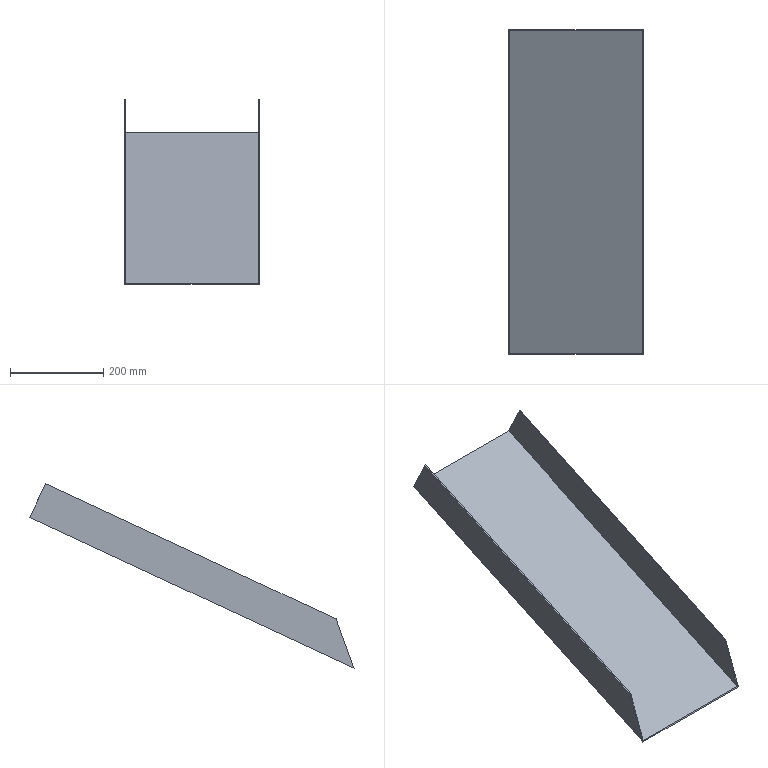Part | NX | features solid 2 | 1 solid | 10 faces | box 290 x 696.58 x 397.325 mm | volume 672211 mm3 | plane 10
STEP:
#1=CARTESIAN_POINT('',(310.,-279.682,-230.));
#2=VERTEX_POINT('',#1);
#3=CARTESIAN_POINT('',(310.,-976.262,-554.821));
#4=VERTEX_POINT('',#3);
#5=CARTESIAN_POINT('',(310.,235.,10.));
#6=DIRECTION('',(0.,-0.9063,-0.4226));
#7=VECTOR('',#6,1000.);
#8=LINE('',#5,#7);
#9=EDGE_CURVE('',#2,#4,#8,.T.);
#10=ORIENTED_EDGE('',*,*,#9,.F.);
#11=CARTESIAN_POINT('',(310.,-313.491,-157.495));
#12=VERTEX_POINT('',#11);
#13=CARTESIAN_POINT('',(310.,-300.813,-184.685));
#14=DIRECTION('',(0.,-0.4226,0.9063));
#15=VECTOR('',#14,1000.);
#16=LINE('',#13,#15);
#17=EDGE_CURVE('',#2,#12,#16,.T.);
#18=ORIENTED_EDGE('',*,*,#17,.T.);
#19=CARTESIAN_POINT('',(310.,-937.566,-448.506));
#20=VERTEX_POINT('',#19);
#21=CARTESIAN_POINT('',(310.,201.191,82.505));
#22=DIRECTION('',(0.,-0.9063,-0.4226));
#23=VECTOR('',#22,1000.);
#24=LINE('',#21,#23);
#25=EDGE_CURVE('',#12,#20,#24,.T.);
#26=ORIENTED_EDGE('',*,*,#25,.T.);
#27=CARTESIAN_POINT('',(310.,-937.566,-448.506));
#28=DIRECTION('',(0.,-0.342,-0.9397));
#29=VECTOR('',#28,1000.);
#30=LINE('',#27,#29);
#31=EDGE_CURVE('',#4,#20,#30,.F.);
#32=ORIENTED_EDGE('',*,*,#31,.F.);
#33=EDGE_LOOP('',(#10,#18,#26,#32));
#34=FACE_BOUND('',#33,.T.);
#35=CARTESIAN_POINT('',(310.,0.,0.));
#36=DIRECTION('',(1.,0.,0.));
#37=DIRECTION('',(0.,0.,-1.));
#38=AXIS2_PLACEMENT_3D('',#35,#36,#37);
#39=PLANE('',#38);
#40=ADVANCED_FACE('',(#34),#39,.T.);
#41=CARTESIAN_POINT('',(308.,-280.527,-228.187));
#42=VERTEX_POINT('',#41);
#43=CARTESIAN_POINT('',(22.,-280.527,-228.187));
#44=VERTEX_POINT('',#43);
#45=CARTESIAN_POINT('',(290.,-280.527,-228.187));
#46=DIRECTION('',(-1.,0.,0.));
#47=VECTOR('',#46,1000.);
#48=LINE('',#45,#47);
#49=EDGE_CURVE('',#42,#44,#48,.T.);
#50=ORIENTED_EDGE('',*,*,#49,.F.);
#51=CARTESIAN_POINT('',(308.,-313.491,-157.495));
#52=VERTEX_POINT('',#51);
#53=CARTESIAN_POINT('',(308.,-300.813,-184.685));
#54=DIRECTION('',(0.,0.4226,-0.9063));
#55=VECTOR('',#54,1000.);
#56=LINE('',#53,#55);
#57=EDGE_CURVE('',#52,#42,#56,.T.);
#58=ORIENTED_EDGE('',*,*,#57,.F.);
#59=CARTESIAN_POINT('',(40.,-313.491,-157.495));
#60=DIRECTION('',(1.,0.,0.));
#61=VECTOR('',#60,1000.);
#62=LINE('',#59,#61);
#63=EDGE_CURVE('',#52,#12,#62,.T.);
#64=ORIENTED_EDGE('',*,*,#63,.T.);
#65=ORIENTED_EDGE('',*,*,#17,.F.);
#66=CARTESIAN_POINT('',(20.,-279.682,-230.));
#67=VERTEX_POINT('',#66);
#68=CARTESIAN_POINT('',(1490.,-279.682,-230.));
#69=DIRECTION('',(-1.,0.,0.));
#70=VECTOR('',#69,1000.);
#71=LINE('',#68,#70);
#72=EDGE_CURVE('',#2,#67,#71,.T.);
#73=ORIENTED_EDGE('',*,*,#72,.T.);
#74=CARTESIAN_POINT('',(20.,-313.491,-157.495));
#75=VERTEX_POINT('',#74);
#76=CARTESIAN_POINT('',(20.,-300.813,-184.685));
#77=DIRECTION('',(0.,0.4226,-0.9063));
#78=VECTOR('',#77,1000.);
#79=LINE('',#76,#78);
#80=EDGE_CURVE('',#75,#67,#79,.T.);
#81=ORIENTED_EDGE('',*,*,#80,.F.);
#82=CARTESIAN_POINT('',(22.,-313.491,-157.495));
#83=VERTEX_POINT('',#82);
#84=CARTESIAN_POINT('',(290.,-313.491,-157.495));
#85=DIRECTION('',(-1.,0.,0.));
#86=VECTOR('',#85,1000.);
#87=LINE('',#84,#86);
#88=EDGE_CURVE('',#83,#75,#87,.T.);
#89=ORIENTED_EDGE('',*,*,#88,.F.);
#90=CARTESIAN_POINT('',(22.,-300.813,-184.685));
#91=DIRECTION('',(0.,0.4226,-0.9063));
#92=VECTOR('',#91,1000.);
#93=LINE('',#90,#92);
#94=EDGE_CURVE('',#83,#44,#93,.T.);
#95=ORIENTED_EDGE('',*,*,#94,.T.);
#96=EDGE_LOOP('',(#50,#58,#64,#65,#73,#81,#89,#95));
#97=FACE_BOUND('',#96,.T.);
#98=CARTESIAN_POINT('',(1490.,-300.813,-184.685));
#99=DIRECTION('',(0.,-0.9063,-0.4226));
#100=DIRECTION('',(0.,0.4226,-0.9063));
#101=AXIS2_PLACEMENT_3D('',#98,#99,#100);
#102=PLANE('',#101);
#103=ADVANCED_FACE('',(#97),#102,.F.);
#104=ORIENTED_EDGE('',*,*,#72,.F.);
#105=ORIENTED_EDGE('',*,*,#9,.T.);
#106=CARTESIAN_POINT('',(20.,-976.262,-554.821));
#107=VERTEX_POINT('',#106);
#108=CARTESIAN_POINT('',(290.,-976.262,-554.821));
#109=DIRECTION('',(1.,0.,0.));
#110=VECTOR('',#109,1000.);
#111=LINE('',#108,#110);
#112=EDGE_CURVE('',#107,#4,#111,.T.);
#113=ORIENTED_EDGE('',*,*,#112,.F.);
#114=CARTESIAN_POINT('',(20.,235.,10.));
#115=DIRECTION('',(0.,-0.9063,-0.4226));
#116=VECTOR('',#115,1000.);
#117=LINE('',#114,#116);
#118=EDGE_CURVE('',#67,#107,#117,.T.);
#119=ORIENTED_EDGE('',*,*,#118,.F.);
#120=EDGE_LOOP('',(#104,#105,#113,#119));
#121=FACE_BOUND('',#120,.T.);
#122=CARTESIAN_POINT('',(290.,235.,10.));
#123=DIRECTION('',(0.,0.4226,-0.9063));
#124=DIRECTION('',(0.,-0.9063,-0.4226));
#125=AXIS2_PLACEMENT_3D('',#122,#123,#124);
#126=PLANE('',#125);
#127=ADVANCED_FACE('',(#121),#126,.T.);
#128=ORIENTED_EDGE('',*,*,#49,.T.);
#129=CARTESIAN_POINT('',(22.,-975.294,-552.163));
#130=VERTEX_POINT('',#129);
#131=CARTESIAN_POINT('',(22.,234.155,11.813));
#132=DIRECTION('',(0.,-0.9063,-0.4226));
#133=VECTOR('',#132,1000.);
#134=LINE('',#131,#133);
#135=EDGE_CURVE('',#44,#130,#134,.T.);
#136=ORIENTED_EDGE('',*,*,#135,.T.);
#137=CARTESIAN_POINT('',(308.,-975.294,-552.163));
#138=VERTEX_POINT('',#137);
#139=CARTESIAN_POINT('',(290.,-975.294,-552.163));
#140=DIRECTION('',(-1.,0.,0.));
#141=VECTOR('',#140,1000.);
#142=LINE('',#139,#141);
#143=EDGE_CURVE('',#130,#138,#142,.F.);
#144=ORIENTED_EDGE('',*,*,#143,.T.);
#145=CARTESIAN_POINT('',(308.,234.155,11.813));
#146=DIRECTION('',(0.,-0.9063,-0.4226));
#147=VECTOR('',#146,1000.);
#148=LINE('',#145,#147);
#149=EDGE_CURVE('',#42,#138,#148,.T.);
#150=ORIENTED_EDGE('',*,*,#149,.F.);
#151=EDGE_LOOP('',(#128,#136,#144,#150));
#152=FACE_BOUND('',#151,.T.);
#153=CARTESIAN_POINT('',(290.,234.155,11.813));
#154=DIRECTION('',(0.,0.4226,-0.9063));
#155=DIRECTION('',(0.,-0.9063,-0.4226));
#156=AXIS2_PLACEMENT_3D('',#153,#154,#155);
#157=PLANE('',#156);
#158=ADVANCED_FACE('',(#152),#157,.F.);
#159=CARTESIAN_POINT('',(20.,-937.566,-448.506));
#160=VERTEX_POINT('',#159);
#161=CARTESIAN_POINT('',(20.,-937.566,-448.506));
#162=DIRECTION('',(0.,-0.342,-0.9397));
#163=VECTOR('',#162,1000.);
#164=LINE('',#161,#163);
#165=EDGE_CURVE('',#107,#160,#164,.F.);
#166=ORIENTED_EDGE('',*,*,#165,.F.);
#167=ORIENTED_EDGE('',*,*,#112,.T.);
#168=ORIENTED_EDGE('',*,*,#31,.T.);
#169=CARTESIAN_POINT('',(308.,-937.566,-448.506));
#170=VERTEX_POINT('',#169);
#171=CARTESIAN_POINT('',(40.,-937.566,-448.506));
#172=DIRECTION('',(1.,0.,0.));
#173=VECTOR('',#172,1000.);
#174=LINE('',#171,#173);
#175=EDGE_CURVE('',#20,#170,#174,.F.);
#176=ORIENTED_EDGE('',*,*,#175,.T.);
#177=CARTESIAN_POINT('',(308.,-640.949,366.444));
#178=DIRECTION('',(0.,0.342,0.9397));
#179=VECTOR('',#178,1000.);
#180=LINE('',#177,#179);
#181=EDGE_CURVE('',#170,#138,#180,.F.);
#182=ORIENTED_EDGE('',*,*,#181,.T.);
#183=ORIENTED_EDGE('',*,*,#143,.F.);
#184=CARTESIAN_POINT('',(22.,-937.566,-448.506));
#185=VERTEX_POINT('',#184);
#186=CARTESIAN_POINT('',(22.,-640.949,366.444));
#187=DIRECTION('',(0.,0.342,0.9397));
#188=VECTOR('',#187,1000.);
#189=LINE('',#186,#188);
#190=EDGE_CURVE('',#185,#130,#189,.F.);
#191=ORIENTED_EDGE('',*,*,#190,.F.);
#192=CARTESIAN_POINT('',(290.,-937.566,-448.506));
#193=DIRECTION('',(-1.,0.,0.));
#194=VECTOR('',#193,1000.);
#195=LINE('',#192,#194);
#196=EDGE_CURVE('',#160,#185,#195,.F.);
#197=ORIENTED_EDGE('',*,*,#196,.F.);
#198=EDGE_LOOP('',(#166,#167,#168,#176,#182,#183,#191,#197));
#199=FACE_BOUND('',#198,.T.);
#200=CARTESIAN_POINT('',(290.,-937.566,-448.506));
#201=DIRECTION('',(0.,0.9397,-0.342));
#202=DIRECTION('',(0.,0.342,0.9397));
#203=AXIS2_PLACEMENT_3D('',#200,#201,#202);
#204=PLANE('',#203);
#205=ADVANCED_FACE('',(#199),#204,.F.);
#206=CARTESIAN_POINT('',(20.,201.191,82.505));
#207=DIRECTION('',(0.,-0.9063,-0.4226));
#208=VECTOR('',#207,1000.);
#209=LINE('',#206,#208);
#210=EDGE_CURVE('',#75,#160,#209,.T.);
#211=ORIENTED_EDGE('',*,*,#210,.T.);
#212=ORIENTED_EDGE('',*,*,#196,.T.);
#213=CARTESIAN_POINT('',(22.,201.191,82.505));
#214=DIRECTION('',(0.,-0.9063,-0.4226));
#215=VECTOR('',#214,1000.);
#216=LINE('',#213,#215);
#217=EDGE_CURVE('',#83,#185,#216,.T.);
#218=ORIENTED_EDGE('',*,*,#217,.F.);
#219=ORIENTED_EDGE('',*,*,#88,.T.);
#220=EDGE_LOOP('',(#211,#212,#218,#219));
#221=FACE_BOUND('',#220,.T.);
#222=CARTESIAN_POINT('',(290.,201.191,82.505));
#223=DIRECTION('',(0.,0.4226,-0.9063));
#224=DIRECTION('',(0.,-0.9063,-0.4226));
#225=AXIS2_PLACEMENT_3D('',#222,#223,#224);
#226=PLANE('',#225);
#227=ADVANCED_FACE('',(#221),#226,.F.);
#228=ORIENTED_EDGE('',*,*,#118,.T.);
#229=ORIENTED_EDGE('',*,*,#165,.T.);
#230=ORIENTED_EDGE('',*,*,#210,.F.);
#231=ORIENTED_EDGE('',*,*,#80,.T.);
#232=EDGE_LOOP('',(#228,#229,#230,#231));
#233=FACE_BOUND('',#232,.T.);
#234=CARTESIAN_POINT('',(20.,213.869,55.315));
#235=DIRECTION('',(1.,0.,0.));
#236=DIRECTION('',(0.,0.,-1.));
#237=AXIS2_PLACEMENT_3D('',#234,#235,#236);
#238=PLANE('',#237);
#239=ADVANCED_FACE('',(#233),#238,.F.);
#240=ORIENTED_EDGE('',*,*,#217,.T.);
#241=ORIENTED_EDGE('',*,*,#190,.T.);
#242=ORIENTED_EDGE('',*,*,#135,.F.);
#243=ORIENTED_EDGE('',*,*,#94,.F.);
#244=EDGE_LOOP('',(#240,#241,#242,#243));
#245=FACE_BOUND('',#244,.T.);
#246=CARTESIAN_POINT('',(22.,213.869,55.315));
#247=DIRECTION('',(1.,0.,0.));
#248=DIRECTION('',(0.,0.,-1.));
#249=AXIS2_PLACEMENT_3D('',#246,#247,#248);
#250=PLANE('',#249);
#251=ADVANCED_FACE('',(#245),#250,.T.);
#252=ORIENTED_EDGE('',*,*,#25,.F.);
#253=ORIENTED_EDGE('',*,*,#63,.F.);
#254=CARTESIAN_POINT('',(308.,201.191,82.505));
#255=DIRECTION('',(0.,-0.9063,-0.4226));
#256=VECTOR('',#255,1000.);
#257=LINE('',#254,#256);
#258=EDGE_CURVE('',#52,#170,#257,.T.);
#259=ORIENTED_EDGE('',*,*,#258,.T.);
#260=ORIENTED_EDGE('',*,*,#175,.F.);
#261=EDGE_LOOP('',(#252,#253,#259,#260));
#262=FACE_BOUND('',#261,.T.);
#263=CARTESIAN_POINT('',(40.,201.191,82.505));
#264=DIRECTION('',(0.,0.4226,-0.9063));
#265=DIRECTION('',(0.,-0.9063,-0.4226));
#266=AXIS2_PLACEMENT_3D('',#263,#264,#265);
#267=PLANE('',#266);
#268=ADVANCED_FACE('',(#262),#267,.F.);
#269=ORIENTED_EDGE('',*,*,#258,.F.);
#270=ORIENTED_EDGE('',*,*,#57,.T.);
#271=ORIENTED_EDGE('',*,*,#149,.T.);
#272=ORIENTED_EDGE('',*,*,#181,.F.);
#273=EDGE_LOOP('',(#269,#270,#271,#272));
#274=FACE_BOUND('',#273,.T.);
#275=CARTESIAN_POINT('',(308.,213.869,55.315));
#276=DIRECTION('',(-1.,0.,0.));
#277=DIRECTION('',(0.,0.,-1.));
#278=AXIS2_PLACEMENT_3D('',#275,#276,#277);
#279=PLANE('',#278);
#280=ADVANCED_FACE('',(#274),#279,.T.);
#281=CLOSED_SHELL('',(#40,#103,#127,#158,#205,#227,#239,#251,#268,#280));
#282=MANIFOLD_SOLID_BREP('',#281);
#283=(LENGTH_UNIT()NAMED_UNIT(*)SI_UNIT(.MILLI.,.METRE.));
#284=UNCERTAINTY_MEASURE_WITH_UNIT(LENGTH_MEASURE(0.00001),#283,'','');
#285=(NAMED_UNIT(*)PLANE_ANGLE_UNIT()SI_UNIT($,.RADIAN.));
#286=(NAMED_UNIT(*)SI_UNIT($,.STERADIAN.)SOLID_ANGLE_UNIT());
#287=(GEOMETRIC_REPRESENTATION_CONTEXT(3)GLOBAL_UNCERTAINTY_ASSIGNED_CONTEXT((#284))GLOBAL_UNIT_ASSIGNED_CONTEXT((#283,#285,#286))REPRESENTATION_CONTEXT('',''));
#288=ADVANCED_BREP_SHAPE_REPRESENTATION('',(#282),#287);